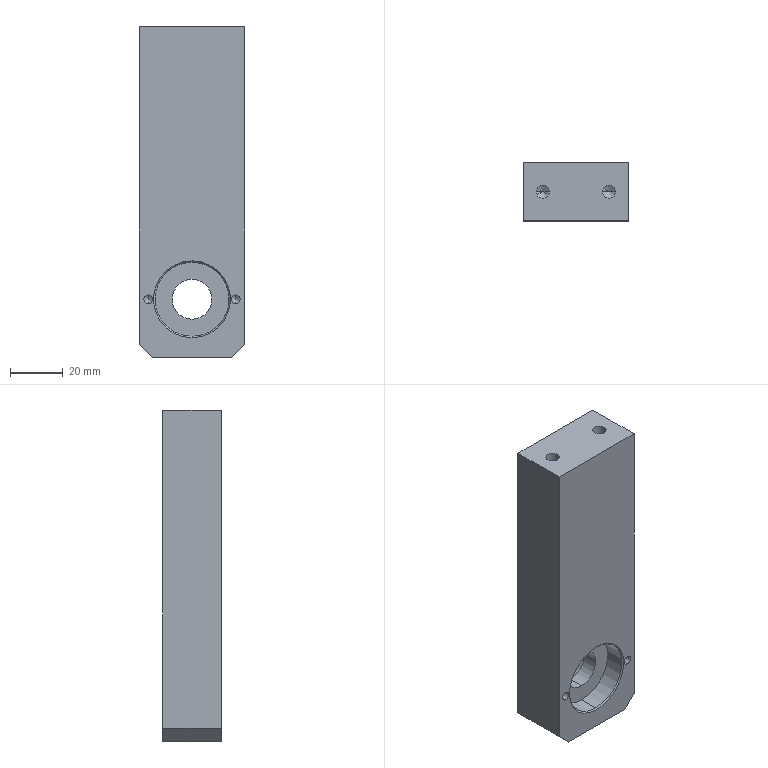Part | SolidWorks | features BaseBody 1 | 1 solid | 44 faces | box 40 x 22 x 125 mm | volume 97550 mm3 | cylinder 18 | cone 16 | plane 10 | commonest cylinder face diameters 3.3 x8 5 x4 28 x4 15 x2
STEP:
#1=CARTESIAN_POINT('',(13.755,11.9,-37.563));
#2=VERTEX_POINT('',#1);
#3=CARTESIAN_POINT('',(13.755,11.9,-34.263));
#4=VERTEX_POINT('',#3);
#5=CARTESIAN_POINT('',(13.755,11.9,-35.913));
#6=DIRECTION('',(0.,1.,0.));
#7=DIRECTION('',(0.,0.,1.));
#8=AXIS2_PLACEMENT_3D('',#5,#6,#7);
#9=CIRCLE('',#8,1.65);
#10=EDGE_CURVE('',#2,#4,#9,.T.);
#11=ORIENTED_EDGE('',*,*,#10,.F.);
#12=CARTESIAN_POINT('',(13.755,22.,-37.563));
#13=VERTEX_POINT('',#12);
#14=CARTESIAN_POINT('',(13.755,22.,-37.563));
#15=DIRECTION('',(0.,1.,0.));
#16=VECTOR('',#15,1000.);
#17=LINE('',#14,#16);
#18=EDGE_CURVE('',#2,#13,#17,.T.);
#19=ORIENTED_EDGE('',*,*,#18,.T.);
#20=CARTESIAN_POINT('',(13.755,22.,-34.263));
#21=VERTEX_POINT('',#20);
#22=CARTESIAN_POINT('',(13.755,22.,-35.913));
#23=DIRECTION('',(0.,1.,0.));
#24=DIRECTION('',(0.,0.,1.));
#25=AXIS2_PLACEMENT_3D('',#22,#23,#24);
#26=CIRCLE('',#25,1.65);
#27=EDGE_CURVE('',#13,#21,#26,.T.);
#28=ORIENTED_EDGE('',*,*,#27,.T.);
#29=CARTESIAN_POINT('',(13.755,22.,-34.263));
#30=DIRECTION('',(0.,1.,0.));
#31=VECTOR('',#30,1000.);
#32=LINE('',#29,#31);
#33=EDGE_CURVE('',#4,#21,#32,.T.);
#34=ORIENTED_EDGE('',*,*,#33,.F.);
#35=EDGE_LOOP('',(#11,#19,#28,#34));
#36=FACE_OUTER_BOUND('',#35,.T.);
#37=CARTESIAN_POINT('',(13.755,22.,-35.913));
#38=DIRECTION('',(0.,1.,0.));
#39=DIRECTION('',(0.,0.,1.));
#40=AXIS2_PLACEMENT_3D('',#37,#38,#39);
#41=CYLINDRICAL_SURFACE('',#40,1.65);
#42=ADVANCED_FACE('',(#36),#41,.F.);
#43=CARTESIAN_POINT('',(13.755,11.,-36.065));
#44=VERTEX_POINT('',#43);
#45=CARTESIAN_POINT('',(13.755,11.,-35.761));
#46=VERTEX_POINT('',#45);
#47=CARTESIAN_POINT('',(13.755,11.,-35.913));
#48=DIRECTION('',(0.,1.,0.));
#49=DIRECTION('',(0.,0.,1.));
#50=AXIS2_PLACEMENT_3D('',#47,#48,#49);
#51=CIRCLE('',#50,0.1521);
#52=EDGE_CURVE('',#44,#46,#51,.T.);
#53=ORIENTED_EDGE('',*,*,#52,.F.);
#54=CARTESIAN_POINT('',(13.755,11.9,-37.563));
#55=DIRECTION('',(0.,0.515,-0.8572));
#56=VECTOR('',#55,1000.);
#57=LINE('',#54,#56);
#58=EDGE_CURVE('',#44,#2,#57,.T.);
#59=ORIENTED_EDGE('',*,*,#58,.T.);
#60=ORIENTED_EDGE('',*,*,#10,.T.);
#61=CARTESIAN_POINT('',(13.755,11.9,-34.263));
#62=DIRECTION('',(0.,0.515,0.8572));
#63=VECTOR('',#62,1000.);
#64=LINE('',#61,#63);
#65=EDGE_CURVE('',#46,#4,#64,.T.);
#66=ORIENTED_EDGE('',*,*,#65,.F.);
#67=EDGE_LOOP('',(#53,#59,#60,#66));
#68=FACE_OUTER_BOUND('',#67,.T.);
#69=CARTESIAN_POINT('',(13.755,11.9,-35.913));
#70=DIRECTION('',(0.,1.,0.));
#71=DIRECTION('',(0.,0.,1.));
#72=AXIS2_PLACEMENT_3D('',#69,#70,#71);
#73=CONICAL_SURFACE('',#72,1.65,1.03);
#74=ADVANCED_FACE('',(#68),#73,.F.);
#75=CARTESIAN_POINT('',(-19.245,11.9,-37.563));
#76=VERTEX_POINT('',#75);
#77=CARTESIAN_POINT('',(-19.245,11.9,-34.263));
#78=VERTEX_POINT('',#77);
#79=CARTESIAN_POINT('',(-19.245,11.9,-35.913));
#80=DIRECTION('',(0.,1.,0.));
#81=DIRECTION('',(0.,0.,1.));
#82=AXIS2_PLACEMENT_3D('',#79,#80,#81);
#83=CIRCLE('',#82,1.65);
#84=EDGE_CURVE('',#76,#78,#83,.T.);
#85=ORIENTED_EDGE('',*,*,#84,.F.);
#86=CARTESIAN_POINT('',(-19.245,22.,-37.563));
#87=VERTEX_POINT('',#86);
#88=CARTESIAN_POINT('',(-19.245,22.,-37.563));
#89=DIRECTION('',(0.,1.,0.));
#90=VECTOR('',#89,1000.);
#91=LINE('',#88,#90);
#92=EDGE_CURVE('',#76,#87,#91,.T.);
#93=ORIENTED_EDGE('',*,*,#92,.T.);
#94=CARTESIAN_POINT('',(-19.245,22.,-34.263));
#95=VERTEX_POINT('',#94);
#96=CARTESIAN_POINT('',(-19.245,22.,-35.913));
#97=DIRECTION('',(0.,1.,0.));
#98=DIRECTION('',(0.,0.,1.));
#99=AXIS2_PLACEMENT_3D('',#96,#97,#98);
#100=CIRCLE('',#99,1.65);
#101=EDGE_CURVE('',#87,#95,#100,.T.);
#102=ORIENTED_EDGE('',*,*,#101,.T.);
#103=CARTESIAN_POINT('',(-19.245,22.,-34.263));
#104=DIRECTION('',(0.,1.,0.));
#105=VECTOR('',#104,1000.);
#106=LINE('',#103,#105);
#107=EDGE_CURVE('',#78,#95,#106,.T.);
#108=ORIENTED_EDGE('',*,*,#107,.F.);
#109=EDGE_LOOP('',(#85,#93,#102,#108));
#110=FACE_OUTER_BOUND('',#109,.T.);
#111=CARTESIAN_POINT('',(-19.245,22.,-35.913));
#112=DIRECTION('',(0.,1.,0.));
#113=DIRECTION('',(0.,0.,1.));
#114=AXIS2_PLACEMENT_3D('',#111,#112,#113);
#115=CYLINDRICAL_SURFACE('',#114,1.65);
#116=ADVANCED_FACE('',(#110),#115,.F.);
#117=CARTESIAN_POINT('',(-19.245,11.,-36.065));
#118=VERTEX_POINT('',#117);
#119=CARTESIAN_POINT('',(-19.245,11.,-35.761));
#120=VERTEX_POINT('',#119);
#121=CARTESIAN_POINT('',(-19.245,11.,-35.913));
#122=DIRECTION('',(0.,1.,0.));
#123=DIRECTION('',(0.,0.,1.));
#124=AXIS2_PLACEMENT_3D('',#121,#122,#123);
#125=CIRCLE('',#124,0.1521);
#126=EDGE_CURVE('',#118,#120,#125,.T.);
#127=ORIENTED_EDGE('',*,*,#126,.F.);
#128=CARTESIAN_POINT('',(-19.245,11.9,-37.563));
#129=DIRECTION('',(0.,0.515,-0.8572));
#130=VECTOR('',#129,1000.);
#131=LINE('',#128,#130);
#132=EDGE_CURVE('',#118,#76,#131,.T.);
#133=ORIENTED_EDGE('',*,*,#132,.T.);
#134=ORIENTED_EDGE('',*,*,#84,.T.);
#135=CARTESIAN_POINT('',(-19.245,11.9,-34.263));
#136=DIRECTION('',(0.,0.515,0.8572));
#137=VECTOR('',#136,1000.);
#138=LINE('',#135,#137);
#139=EDGE_CURVE('',#120,#78,#138,.T.);
#140=ORIENTED_EDGE('',*,*,#139,.F.);
#141=EDGE_LOOP('',(#127,#133,#134,#140));
#142=FACE_OUTER_BOUND('',#141,.T.);
#143=CARTESIAN_POINT('',(-19.245,11.9,-35.913));
#144=DIRECTION('',(0.,1.,0.));
#145=DIRECTION('',(0.,0.,1.));
#146=AXIS2_PLACEMENT_3D('',#143,#144,#145);
#147=CONICAL_SURFACE('',#146,1.65,1.03);
#148=ADVANCED_FACE('',(#142),#147,.F.);
#149=CARTESIAN_POINT('',(13.755,10.1,-34.263));
#150=VERTEX_POINT('',#149);
#151=CARTESIAN_POINT('',(13.755,10.1,-37.563));
#152=VERTEX_POINT('',#151);
#153=CARTESIAN_POINT('',(13.755,10.1,-35.913));
#154=DIRECTION('',(0.,-1.,0.));
#155=DIRECTION('',(0.,0.,-1.));
#156=AXIS2_PLACEMENT_3D('',#153,#154,#155);
#157=CIRCLE('',#156,1.65);
#158=EDGE_CURVE('',#150,#152,#157,.T.);
#159=ORIENTED_EDGE('',*,*,#158,.F.);
#160=CARTESIAN_POINT('',(13.755,0.,-34.263));
#161=VERTEX_POINT('',#160);
#162=CARTESIAN_POINT('',(13.755,0.,-34.263));
#163=DIRECTION('',(0.,-1.,0.));
#164=VECTOR('',#163,1000.);
#165=LINE('',#162,#164);
#166=EDGE_CURVE('',#150,#161,#165,.T.);
#167=ORIENTED_EDGE('',*,*,#166,.T.);
#168=CARTESIAN_POINT('',(13.755,0.,-37.563));
#169=VERTEX_POINT('',#168);
#170=CARTESIAN_POINT('',(13.755,0.,-35.913));
#171=DIRECTION('',(0.,-1.,0.));
#172=DIRECTION('',(0.,0.,-1.));
#173=AXIS2_PLACEMENT_3D('',#170,#171,#172);
#174=CIRCLE('',#173,1.65);
#175=EDGE_CURVE('',#161,#169,#174,.T.);
#176=ORIENTED_EDGE('',*,*,#175,.T.);
#177=CARTESIAN_POINT('',(13.755,0.,-37.563));
#178=DIRECTION('',(0.,-1.,0.));
#179=VECTOR('',#178,1000.);
#180=LINE('',#177,#179);
#181=EDGE_CURVE('',#152,#169,#180,.T.);
#182=ORIENTED_EDGE('',*,*,#181,.F.);
#183=EDGE_LOOP('',(#159,#167,#176,#182));
#184=FACE_OUTER_BOUND('',#183,.T.);
#185=CARTESIAN_POINT('',(13.755,0.,-35.913));
#186=DIRECTION('',(0.,-1.,0.));
#187=DIRECTION('',(0.,0.,-1.));
#188=AXIS2_PLACEMENT_3D('',#185,#186,#187);
#189=CYLINDRICAL_SURFACE('',#188,1.65);
#190=ADVANCED_FACE('',(#184),#189,.F.);
#191=ORIENTED_EDGE('',*,*,#52,.T.);
#192=CARTESIAN_POINT('',(13.755,10.1,-34.263));
#193=DIRECTION('',(0.,-0.515,0.8572));
#194=VECTOR('',#193,1000.);
#195=LINE('',#192,#194);
#196=EDGE_CURVE('',#46,#150,#195,.T.);
#197=ORIENTED_EDGE('',*,*,#196,.T.);
#198=ORIENTED_EDGE('',*,*,#158,.T.);
#199=CARTESIAN_POINT('',(13.755,10.1,-37.563));
#200=DIRECTION('',(0.,-0.515,-0.8572));
#201=VECTOR('',#200,1000.);
#202=LINE('',#199,#201);
#203=EDGE_CURVE('',#44,#152,#202,.T.);
#204=ORIENTED_EDGE('',*,*,#203,.F.);
#205=EDGE_LOOP('',(#191,#197,#198,#204));
#206=FACE_OUTER_BOUND('',#205,.T.);
#207=CARTESIAN_POINT('',(13.755,10.1,-35.913));
#208=DIRECTION('',(0.,-1.,0.));
#209=DIRECTION('',(0.,0.,-1.));
#210=AXIS2_PLACEMENT_3D('',#207,#208,#209);
#211=CONICAL_SURFACE('',#210,1.65,1.03);
#212=ADVANCED_FACE('',(#206),#211,.F.);
#213=CARTESIAN_POINT('',(-19.245,10.1,-34.263));
#214=VERTEX_POINT('',#213);
#215=CARTESIAN_POINT('',(-19.245,10.1,-37.563));
#216=VERTEX_POINT('',#215);
#217=CARTESIAN_POINT('',(-19.245,10.1,-35.913));
#218=DIRECTION('',(0.,-1.,0.));
#219=DIRECTION('',(0.,0.,-1.));
#220=AXIS2_PLACEMENT_3D('',#217,#218,#219);
#221=CIRCLE('',#220,1.65);
#222=EDGE_CURVE('',#214,#216,#221,.T.);
#223=ORIENTED_EDGE('',*,*,#222,.F.);
#224=CARTESIAN_POINT('',(-19.245,0.,-34.263));
#225=VERTEX_POINT('',#224);
#226=CARTESIAN_POINT('',(-19.245,0.,-34.263));
#227=DIRECTION('',(0.,-1.,0.));
#228=VECTOR('',#227,1000.);
#229=LINE('',#226,#228);
#230=EDGE_CURVE('',#214,#225,#229,.T.);
#231=ORIENTED_EDGE('',*,*,#230,.T.);
#232=CARTESIAN_POINT('',(-19.245,0.,-37.563));
#233=VERTEX_POINT('',#232);
#234=CARTESIAN_POINT('',(-19.245,0.,-35.913));
#235=DIRECTION('',(0.,-1.,0.));
#236=DIRECTION('',(0.,0.,-1.));
#237=AXIS2_PLACEMENT_3D('',#234,#235,#236);
#238=CIRCLE('',#237,1.65);
#239=EDGE_CURVE('',#225,#233,#238,.T.);
#240=ORIENTED_EDGE('',*,*,#239,.T.);
#241=CARTESIAN_POINT('',(-19.245,0.,-37.563));
#242=DIRECTION('',(0.,-1.,0.));
#243=VECTOR('',#242,1000.);
#244=LINE('',#241,#243);
#245=EDGE_CURVE('',#216,#233,#244,.T.);
#246=ORIENTED_EDGE('',*,*,#245,.F.);
#247=EDGE_LOOP('',(#223,#231,#240,#246));
#248=FACE_OUTER_BOUND('',#247,.T.);
#249=CARTESIAN_POINT('',(-19.245,0.,-35.913));
#250=DIRECTION('',(0.,-1.,0.));
#251=DIRECTION('',(0.,0.,-1.));
#252=AXIS2_PLACEMENT_3D('',#249,#250,#251);
#253=CYLINDRICAL_SURFACE('',#252,1.65);
#254=ADVANCED_FACE('',(#248),#253,.F.);
#255=ORIENTED_EDGE('',*,*,#126,.T.);
#256=CARTESIAN_POINT('',(-19.245,10.1,-34.263));
#257=DIRECTION('',(0.,-0.515,0.8572));
#258=VECTOR('',#257,1000.);
#259=LINE('',#256,#258);
#260=EDGE_CURVE('',#120,#214,#259,.T.);
#261=ORIENTED_EDGE('',*,*,#260,.T.);
#262=ORIENTED_EDGE('',*,*,#222,.T.);
#263=CARTESIAN_POINT('',(-19.245,10.1,-37.563));
#264=DIRECTION('',(0.,-0.515,-0.8572));
#265=VECTOR('',#264,1000.);
#266=LINE('',#263,#265);
#267=EDGE_CURVE('',#118,#216,#266,.T.);
#268=ORIENTED_EDGE('',*,*,#267,.F.);
#269=EDGE_LOOP('',(#255,#261,#262,#268));
#270=FACE_OUTER_BOUND('',#269,.T.);
#271=CARTESIAN_POINT('',(-19.245,10.1,-35.913));
#272=DIRECTION('',(0.,-1.,0.));
#273=DIRECTION('',(0.,0.,-1.));
#274=AXIS2_PLACEMENT_3D('',#271,#272,#273);
#275=CONICAL_SURFACE('',#274,1.65,1.03);
#276=ADVANCED_FACE('',(#270),#275,.F.);
#277=CARTESIAN_POINT('',(-2.745,0.5,-21.913));
#278=VERTEX_POINT('',#277);
#279=CARTESIAN_POINT('',(-2.745,0.5,-49.913));
#280=VERTEX_POINT('',#279);
#281=CARTESIAN_POINT('',(-2.745,0.5,-35.913));
#282=DIRECTION('',(0.,-1.,0.));
#283=DIRECTION('',(0.,0.,1.));
#284=AXIS2_PLACEMENT_3D('',#281,#282,#283);
#285=CIRCLE('',#284,14.);
#286=EDGE_CURVE('',#278,#280,#285,.T.);
#287=ORIENTED_EDGE('',*,*,#286,.F.);
#288=CARTESIAN_POINT('',(-2.745,0.,-21.413));
#289=VERTEX_POINT('',#288);
#290=CARTESIAN_POINT('',(-2.745,0.5,-21.913));
#291=DIRECTION('',(0.,-0.7071,0.7071));
#292=VECTOR('',#291,1000.);
#293=LINE('',#290,#292);
#294=EDGE_CURVE('',#278,#289,#293,.T.);
#295=ORIENTED_EDGE('',*,*,#294,.T.);
#296=CARTESIAN_POINT('',(-2.745,0.,-50.413));
#297=VERTEX_POINT('',#296);
#298=CARTESIAN_POINT('',(-2.745,0.,-35.913));
#299=DIRECTION('',(0.,1.,0.));
#300=DIRECTION('',(0.,0.,1.));
#301=AXIS2_PLACEMENT_3D('',#298,#299,#300);
#302=CIRCLE('',#301,14.5);
#303=EDGE_CURVE('',#297,#289,#302,.T.);
#304=ORIENTED_EDGE('',*,*,#303,.F.);
#305=CARTESIAN_POINT('',(-2.745,0.5,-49.913));
#306=DIRECTION('',(0.,-0.7071,-0.7071));
#307=VECTOR('',#306,1000.);
#308=LINE('',#305,#307);
#309=EDGE_CURVE('',#280,#297,#308,.T.);
#310=ORIENTED_EDGE('',*,*,#309,.F.);
#311=EDGE_LOOP('',(#287,#295,#304,#310));
#312=FACE_OUTER_BOUND('',#311,.T.);
#313=CARTESIAN_POINT('',(-2.745,0.5,-35.913));
#314=DIRECTION('',(0.,-1.,0.));
#315=DIRECTION('',(0.,0.,-1.));
#316=AXIS2_PLACEMENT_3D('',#313,#314,#315);
#317=CONICAL_SURFACE('',#316,14.,0.7854);
#318=ADVANCED_FACE('',(#312),#317,.F.);
#319=CARTESIAN_POINT('',(-2.745,21.5,-49.913));
#320=VERTEX_POINT('',#319);
#321=CARTESIAN_POINT('',(-2.745,21.5,-21.913));
#322=VERTEX_POINT('',#321);
#323=CARTESIAN_POINT('',(-2.745,21.5,-35.913));
#324=DIRECTION('',(0.,1.,0.));
#325=DIRECTION('',(0.,0.,1.));
#326=AXIS2_PLACEMENT_3D('',#323,#324,#325);
#327=CIRCLE('',#326,14.);
#328=EDGE_CURVE('',#320,#322,#327,.T.);
#329=ORIENTED_EDGE('',*,*,#328,.F.);
#330=CARTESIAN_POINT('',(-2.745,22.,-50.413));
#331=VERTEX_POINT('',#330);
#332=CARTESIAN_POINT('',(-2.745,21.5,-49.913));
#333=DIRECTION('',(0.,0.7071,-0.7071));
#334=VECTOR('',#333,1000.);
#335=LINE('',#332,#334);
#336=EDGE_CURVE('',#320,#331,#335,.T.);
#337=ORIENTED_EDGE('',*,*,#336,.T.);
#338=CARTESIAN_POINT('',(-2.745,22.,-21.413));
#339=VERTEX_POINT('',#338);
#340=CARTESIAN_POINT('',(-2.745,22.,-35.913));
#341=DIRECTION('',(0.,-1.,0.));
#342=DIRECTION('',(0.,0.,1.));
#343=AXIS2_PLACEMENT_3D('',#340,#341,#342);
#344=CIRCLE('',#343,14.5);
#345=EDGE_CURVE('',#339,#331,#344,.T.);
#346=ORIENTED_EDGE('',*,*,#345,.F.);
#347=CARTESIAN_POINT('',(-2.745,21.5,-21.913));
#348=DIRECTION('',(0.,0.7071,0.7071));
#349=VECTOR('',#348,1000.);
#350=LINE('',#347,#349);
#351=EDGE_CURVE('',#322,#339,#350,.T.);
#352=ORIENTED_EDGE('',*,*,#351,.F.);
#353=EDGE_LOOP('',(#329,#337,#346,#352));
#354=FACE_OUTER_BOUND('',#353,.T.);
#355=CARTESIAN_POINT('',(-2.745,21.5,-35.913));
#356=DIRECTION('',(0.,1.,0.));
#357=DIRECTION('',(0.,0.,1.));
#358=AXIS2_PLACEMENT_3D('',#355,#356,#357);
#359=CONICAL_SURFACE('',#358,14.,0.7854);
#360=ADVANCED_FACE('',(#354),#359,.F.);
#361=CARTESIAN_POINT('',(-2.745,8.,-21.913));
#362=VERTEX_POINT('',#361);
#363=CARTESIAN_POINT('',(-2.745,8.,-49.913));
#364=VERTEX_POINT('',#363);
#365=CARTESIAN_POINT('',(-2.745,8.,-35.913));
#366=DIRECTION('',(0.,-1.,0.));
#367=DIRECTION('',(0.,0.,-1.));
#368=AXIS2_PLACEMENT_3D('',#365,#366,#367);
#369=CIRCLE('',#368,14.);
#370=EDGE_CURVE('',#362,#364,#369,.T.);
#371=ORIENTED_EDGE('',*,*,#370,.F.);
#372=CARTESIAN_POINT('',(-2.745,8.,-21.913));
#373=DIRECTION('',(0.,-1.,0.));
#374=VECTOR('',#373,1000.);
#375=LINE('',#372,#374);
#376=EDGE_CURVE('',#362,#278,#375,.T.);
#377=ORIENTED_EDGE('',*,*,#376,.T.);
#378=ORIENTED_EDGE('',*,*,#286,.T.);
#379=CARTESIAN_POINT('',(-2.745,8.,-49.913));
#380=DIRECTION('',(0.,-1.,0.));
#381=VECTOR('',#380,1000.);
#382=LINE('',#379,#381);
#383=EDGE_CURVE('',#364,#280,#382,.T.);
#384=ORIENTED_EDGE('',*,*,#383,.F.);
#385=EDGE_LOOP('',(#371,#377,#378,#384));
#386=FACE_OUTER_BOUND('',#385,.T.);
#387=CARTESIAN_POINT('',(-2.745,8.,-35.913));
#388=DIRECTION('',(0.,-1.,0.));
#389=DIRECTION('',(0.,0.,-1.));
#390=AXIS2_PLACEMENT_3D('',#387,#388,#389);
#391=CYLINDRICAL_SURFACE('',#390,14.);
#392=ADVANCED_FACE('',(#386),#391,.F.);
#393=CARTESIAN_POINT('',(-17.745,11.,52.087));
#394=VERTEX_POINT('',#393);
#395=CARTESIAN_POINT('',(-12.745,11.,52.087));
#396=VERTEX_POINT('',#395);
#397=CARTESIAN_POINT('',(-15.245,11.,52.087));
#398=DIRECTION('',(0.,0.,1.));
#399=DIRECTION('',(1.,0.,0.));
#400=AXIS2_PLACEMENT_3D('',#397,#398,#399);
#401=CIRCLE('',#400,2.5);
#402=EDGE_CURVE('',#394,#396,#401,.T.);
#403=ORIENTED_EDGE('',*,*,#402,.F.);
#404=CARTESIAN_POINT('',(-17.745,11.,67.087));
#405=VERTEX_POINT('',#404);
#406=CARTESIAN_POINT('',(-17.745,11.,67.087));
#407=DIRECTION('',(0.,0.,1.));
#408=VECTOR('',#407,1000.);
#409=LINE('',#406,#408);
#410=EDGE_CURVE('',#394,#405,#409,.T.);
#411=ORIENTED_EDGE('',*,*,#410,.T.);
#412=CARTESIAN_POINT('',(-12.745,11.,67.087));
#413=VERTEX_POINT('',#412);
#414=CARTESIAN_POINT('',(-15.245,11.,67.087));
#415=DIRECTION('',(0.,0.,1.));
#416=DIRECTION('',(1.,0.,0.));
#417=AXIS2_PLACEMENT_3D('',#414,#415,#416);
#418=CIRCLE('',#417,2.5);
#419=EDGE_CURVE('',#405,#413,#418,.T.);
#420=ORIENTED_EDGE('',*,*,#419,.T.);
#421=CARTESIAN_POINT('',(-12.745,11.,67.087));
#422=DIRECTION('',(0.,0.,1.));
#423=VECTOR('',#422,1000.);
#424=LINE('',#421,#423);
#425=EDGE_CURVE('',#396,#413,#424,.T.);
#426=ORIENTED_EDGE('',*,*,#425,.F.);
#427=EDGE_LOOP('',(#403,#411,#420,#426));
#428=FACE_OUTER_BOUND('',#427,.T.);
#429=CARTESIAN_POINT('',(-15.245,11.,67.087));
#430=DIRECTION('',(0.,0.,1.));
#431=DIRECTION('',(1.,0.,0.));
#432=AXIS2_PLACEMENT_3D('',#429,#430,#431);
#433=CYLINDRICAL_SURFACE('',#432,2.5);
#434=ADVANCED_FACE('',(#428),#433,.F.);
#435=CARTESIAN_POINT('',(-15.245,11.,50.585));
#436=VERTEX_POINT('',#435);
#437=CARTESIAN_POINT('',(-12.745,11.,52.087));
#438=DIRECTION('',(0.8572,0.,0.515));
#439=VECTOR('',#438,1000.);
#440=LINE('',#437,#439);
#441=EDGE_CURVE('',#436,#396,#440,.T.);
#442=ORIENTED_EDGE('',*,*,#441,.F.);
#443=CARTESIAN_POINT('',(-17.745,11.,52.087));
#444=DIRECTION('',(-0.8572,0.,0.515));
#445=VECTOR('',#444,1000.);
#446=LINE('',#443,#445);
#447=EDGE_CURVE('',#436,#394,#446,.T.);
#448=ORIENTED_EDGE('',*,*,#447,.T.);
#449=ORIENTED_EDGE('',*,*,#402,.T.);
#450=EDGE_LOOP('',(#442,#448,#449));
#451=FACE_OUTER_BOUND('',#450,.T.);
#452=CARTESIAN_POINT('',(-15.245,11.,52.087));
#453=DIRECTION('',(0.,0.,1.));
#454=DIRECTION('',(1.,0.,0.));
#455=AXIS2_PLACEMENT_3D('',#452,#453,#454);
#456=CONICAL_SURFACE('',#455,2.5,1.03);
#457=ADVANCED_FACE('',(#451),#456,.F.);
#458=CARTESIAN_POINT('',(7.255,11.,52.087));
#459=VERTEX_POINT('',#458);
#460=CARTESIAN_POINT('',(12.255,11.,52.087));
#461=VERTEX_POINT('',#460);
#462=CARTESIAN_POINT('',(9.755,11.,52.087));
#463=DIRECTION('',(0.,0.,1.));
#464=DIRECTION('',(1.,0.,0.));
#465=AXIS2_PLACEMENT_3D('',#462,#463,#464);
#466=CIRCLE('',#465,2.5);
#467=EDGE_CURVE('',#459,#461,#466,.T.);
#468=ORIENTED_EDGE('',*,*,#467,.F.);
#469=CARTESIAN_POINT('',(7.255,11.,67.087));
#470=VERTEX_POINT('',#469);
#471=CARTESIAN_POINT('',(7.255,11.,67.087));
#472=DIRECTION('',(0.,0.,1.));
#473=VECTOR('',#472,1000.);
#474=LINE('',#471,#473);
#475=EDGE_CURVE('',#459,#470,#474,.T.);
#476=ORIENTED_EDGE('',*,*,#475,.T.);
#477=CARTESIAN_POINT('',(12.255,11.,67.087));
#478=VERTEX_POINT('',#477);
#479=CARTESIAN_POINT('',(9.755,11.,67.087));
#480=DIRECTION('',(0.,0.,1.));
#481=DIRECTION('',(1.,0.,0.));
#482=AXIS2_PLACEMENT_3D('',#479,#480,#481);
#483=CIRCLE('',#482,2.5);
#484=EDGE_CURVE('',#470,#478,#483,.T.);
#485=ORIENTED_EDGE('',*,*,#484,.T.);
#486=CARTESIAN_POINT('',(12.255,11.,67.087));
#487=DIRECTION('',(0.,0.,1.));
#488=VECTOR('',#487,1000.);
#489=LINE('',#486,#488);
#490=EDGE_CURVE('',#461,#478,#489,.T.);
#491=ORIENTED_EDGE('',*,*,#490,.F.);
#492=EDGE_LOOP('',(#468,#476,#485,#491));
#493=FACE_OUTER_BOUND('',#492,.T.);
#494=CARTESIAN_POINT('',(9.755,11.,67.087));
#495=DIRECTION('',(0.,0.,1.));
#496=DIRECTION('',(1.,0.,0.));
#497=AXIS2_PLACEMENT_3D('',#494,#495,#496);
#498=CYLINDRICAL_SURFACE('',#497,2.5);
#499=ADVANCED_FACE('',(#493),#498,.F.);
#500=CARTESIAN_POINT('',(9.755,11.,50.585));
#501=VERTEX_POINT('',#500);
#502=CARTESIAN_POINT('',(12.255,11.,52.087));
#503=DIRECTION('',(0.8572,0.,0.515));
#504=VECTOR('',#503,1000.);
#505=LINE('',#502,#504);
#506=EDGE_CURVE('',#501,#461,#505,.T.);
#507=ORIENTED_EDGE('',*,*,#506,.F.);
#508=CARTESIAN_POINT('',(7.255,11.,52.087));
#509=DIRECTION('',(-0.8572,0.,0.515));
#510=VECTOR('',#509,1000.);
#511=LINE('',#508,#510);
#512=EDGE_CURVE('',#501,#459,#511,.T.);
#513=ORIENTED_EDGE('',*,*,#512,.T.);
#514=ORIENTED_EDGE('',*,*,#467,.T.);
#515=EDGE_LOOP('',(#507,#513,#514));
#516=FACE_OUTER_BOUND('',#515,.T.);
#517=CARTESIAN_POINT('',(9.755,11.,52.087));
#518=DIRECTION('',(0.,0.,1.));
#519=DIRECTION('',(1.,0.,0.));
#520=AXIS2_PLACEMENT_3D('',#517,#518,#519);
#521=CONICAL_SURFACE('',#520,2.5,1.03);
#522=ADVANCED_FACE('',(#516),#521,.F.);
#523=CARTESIAN_POINT('',(-2.745,14.,-49.913));
#524=VERTEX_POINT('',#523);
#525=CARTESIAN_POINT('',(-2.745,14.,-21.913));
#526=VERTEX_POINT('',#525);
#527=CARTESIAN_POINT('',(-2.745,14.,-35.913));
#528=DIRECTION('',(0.,1.,0.));
#529=DIRECTION('',(0.,0.,1.));
#530=AXIS2_PLACEMENT_3D('',#527,#528,#529);
#531=CIRCLE('',#530,14.);
#532=EDGE_CURVE('',#524,#526,#531,.T.);
#533=ORIENTED_EDGE('',*,*,#532,.F.);
#534=CARTESIAN_POINT('',(-2.745,14.,-49.913));
#535=DIRECTION('',(0.,1.,0.));
#536=VECTOR('',#535,1000.);
#537=LINE('',#534,#536);
#538=EDGE_CURVE('',#524,#320,#537,.T.);
#539=ORIENTED_EDGE('',*,*,#538,.T.);
#540=ORIENTED_EDGE('',*,*,#328,.T.);
#541=CARTESIAN_POINT('',(-2.745,14.,-21.913));
#542=DIRECTION('',(0.,1.,0.));
#543=VECTOR('',#542,1000.);
#544=LINE('',#541,#543);
#545=EDGE_CURVE('',#526,#322,#544,.T.);
#546=ORIENTED_EDGE('',*,*,#545,.F.);
#547=EDGE_LOOP('',(#533,#539,#540,#546));
#548=FACE_OUTER_BOUND('',#547,.T.);
#549=CARTESIAN_POINT('',(-2.745,14.,-35.913));
#550=DIRECTION('',(0.,1.,0.));
#551=DIRECTION('',(0.,0.,1.));
#552=AXIS2_PLACEMENT_3D('',#549,#550,#551);
#553=CYLINDRICAL_SURFACE('',#552,14.);
#554=ADVANCED_FACE('',(#548),#553,.F.);
#555=CARTESIAN_POINT('',(-2.745,14.,-43.413));
#556=VERTEX_POINT('',#555);
#557=CARTESIAN_POINT('',(-2.745,14.,-28.413));
#558=VERTEX_POINT('',#557);
#559=CARTESIAN_POINT('',(-2.745,14.,-35.913));
#560=DIRECTION('',(0.,1.,0.));
#561=DIRECTION('',(0.,0.,1.));
#562=AXIS2_PLACEMENT_3D('',#559,#560,#561);
#563=CIRCLE('',#562,7.5);
#564=EDGE_CURVE('',#556,#558,#563,.T.);
#565=ORIENTED_EDGE('',*,*,#564,.T.);
#566=CARTESIAN_POINT('',(-2.745,8.,-28.413));
#567=VERTEX_POINT('',#566);
#568=CARTESIAN_POINT('',(-2.745,22.,-28.413));
#569=DIRECTION('',(0.,-1.,0.));
#570=VECTOR('',#569,1000.);
#571=LINE('',#568,#570);
#572=EDGE_CURVE('',#558,#567,#571,.T.);
#573=ORIENTED_EDGE('',*,*,#572,.T.);
#574=CARTESIAN_POINT('',(-2.745,8.,-43.413));
#575=VERTEX_POINT('',#574);
#576=CARTESIAN_POINT('',(-2.745,8.,-35.913));
#577=DIRECTION('',(0.,-1.,0.));
#578=DIRECTION('',(0.,0.,-1.));
#579=AXIS2_PLACEMENT_3D('',#576,#577,#578);
#580=CIRCLE('',#579,7.5);
#581=EDGE_CURVE('',#567,#575,#580,.T.);
#582=ORIENTED_EDGE('',*,*,#581,.T.);
#583=CARTESIAN_POINT('',(-2.745,22.,-43.413));
#584=DIRECTION('',(0.,-1.,0.));
#585=VECTOR('',#584,1000.);
#586=LINE('',#583,#585);
#587=EDGE_CURVE('',#556,#575,#586,.T.);
#588=ORIENTED_EDGE('',*,*,#587,.F.);
#589=EDGE_LOOP('',(#565,#573,#582,#588));
#590=FACE_OUTER_BOUND('',#589,.T.);
#591=CARTESIAN_POINT('',(-2.745,22.,-35.913));
#592=DIRECTION('',(0.,-1.,0.));
#593=DIRECTION('',(0.,0.,-1.));
#594=AXIS2_PLACEMENT_3D('',#591,#592,#593);
#595=CYLINDRICAL_SURFACE('',#594,7.5);
#596=ADVANCED_FACE('',(#590),#595,.F.);
#597=CARTESIAN_POINT('',(-2.745,8.,-35.913));
#598=DIRECTION('',(0.,-1.,0.));
#599=DIRECTION('',(0.,0.,-1.));
#600=AXIS2_PLACEMENT_3D('',#597,#598,#599);
#601=CIRCLE('',#600,7.5);
#602=EDGE_CURVE('',#575,#567,#601,.T.);
#603=ORIENTED_EDGE('',*,*,#602,.F.);
#604=ORIENTED_EDGE('',*,*,#581,.F.);
#605=EDGE_LOOP('',(#603,#604));
#606=FACE_BOUND('',#605,.T.);
#607=CARTESIAN_POINT('',(-2.745,8.,-35.913));
#608=DIRECTION('',(0.,-1.,0.));
#609=DIRECTION('',(0.,0.,-1.));
#610=AXIS2_PLACEMENT_3D('',#607,#608,#609);
#611=CIRCLE('',#610,14.);
#612=EDGE_CURVE('',#364,#362,#611,.T.);
#613=ORIENTED_EDGE('',*,*,#612,.T.);
#614=ORIENTED_EDGE('',*,*,#370,.T.);
#615=EDGE_LOOP('',(#613,#614));
#616=FACE_OUTER_BOUND('',#615,.T.);
#617=CARTESIAN_POINT('',(-2.745,8.,-35.913));
#618=DIRECTION('',(0.,-1.,0.));
#619=DIRECTION('',(0.,0.,-1.));
#620=AXIS2_PLACEMENT_3D('',#617,#618,#619);
#621=PLANE('',#620);
#622=ADVANCED_FACE('',(#606,#616),#621,.T.);
#623=CARTESIAN_POINT('',(-17.745,22.,-57.913));
#624=VERTEX_POINT('',#623);
#625=CARTESIAN_POINT('',(-22.745,22.,-52.913));
#626=VERTEX_POINT('',#625);
#627=CARTESIAN_POINT('',(-37.829,22.,-37.829));
#628=DIRECTION('',(-0.7071,0.,0.7071));
#629=VECTOR('',#628,1000.);
#630=LINE('',#627,#629);
#631=EDGE_CURVE('',#624,#626,#630,.T.);
#632=ORIENTED_EDGE('',*,*,#631,.F.);
#633=CARTESIAN_POINT('',(-17.745,0.,-57.913));
#634=VERTEX_POINT('',#633);
#635=CARTESIAN_POINT('',(-17.745,22.,-57.913));
#636=DIRECTION('',(0.,1.,0.));
#637=VECTOR('',#636,1000.);
#638=LINE('',#635,#637);
#639=EDGE_CURVE('',#634,#624,#638,.T.);
#640=ORIENTED_EDGE('',*,*,#639,.F.);
#641=CARTESIAN_POINT('',(-22.745,0.,-52.913));
#642=VERTEX_POINT('',#641);
#643=CARTESIAN_POINT('',(-22.745,0.,-52.913));
#644=DIRECTION('',(0.7071,0.,-0.7071));
#645=VECTOR('',#644,1000.);
#646=LINE('',#643,#645);
#647=EDGE_CURVE('',#642,#634,#646,.T.);
#648=ORIENTED_EDGE('',*,*,#647,.F.);
#649=CARTESIAN_POINT('',(-22.745,22.,-52.913));
#650=DIRECTION('',(0.,-1.,0.));
#651=VECTOR('',#650,1000.);
#652=LINE('',#649,#651);
#653=EDGE_CURVE('',#626,#642,#652,.T.);
#654=ORIENTED_EDGE('',*,*,#653,.F.);
#655=EDGE_LOOP('',(#632,#640,#648,#654));
#656=FACE_OUTER_BOUND('',#655,.T.);
#657=CARTESIAN_POINT('',(-22.745,22.,-52.913));
#658=DIRECTION('',(0.7071,0.,0.7071));
#659=DIRECTION('',(0.,-1.,0.));
#660=AXIS2_PLACEMENT_3D('',#657,#658,#659);
#661=PLANE('',#660);
#662=ADVANCED_FACE('',(#656),#661,.F.);
#663=CARTESIAN_POINT('',(17.255,22.,-52.913));
#664=VERTEX_POINT('',#663);
#665=CARTESIAN_POINT('',(12.255,22.,-57.913));
#666=VERTEX_POINT('',#665);
#667=CARTESIAN_POINT('',(35.084,22.,-35.084));
#668=DIRECTION('',(-0.7071,0.,-0.7071));
#669=VECTOR('',#668,1000.);
#670=LINE('',#667,#669);
#671=EDGE_CURVE('',#664,#666,#670,.T.);
#672=ORIENTED_EDGE('',*,*,#671,.F.);
#673=CARTESIAN_POINT('',(17.255,0.,-52.913));
#674=VERTEX_POINT('',#673);
#675=CARTESIAN_POINT('',(17.255,22.,-52.913));
#676=DIRECTION('',(0.,1.,0.));
#677=VECTOR('',#676,1000.);
#678=LINE('',#675,#677);
#679=EDGE_CURVE('',#674,#664,#678,.T.);
#680=ORIENTED_EDGE('',*,*,#679,.F.);
#681=CARTESIAN_POINT('',(12.255,0.,-57.913));
#682=VERTEX_POINT('',#681);
#683=CARTESIAN_POINT('',(12.255,0.,-57.913));
#684=DIRECTION('',(0.7071,0.,0.7071));
#685=VECTOR('',#684,1000.);
#686=LINE('',#683,#685);
#687=EDGE_CURVE('',#682,#674,#686,.T.);
#688=ORIENTED_EDGE('',*,*,#687,.F.);
#689=CARTESIAN_POINT('',(12.255,22.,-57.913));
#690=DIRECTION('',(0.,-1.,0.));
#691=VECTOR('',#690,1000.);
#692=LINE('',#689,#691);
#693=EDGE_CURVE('',#666,#682,#692,.T.);
#694=ORIENTED_EDGE('',*,*,#693,.F.);
#695=EDGE_LOOP('',(#672,#680,#688,#694));
#696=FACE_OUTER_BOUND('',#695,.T.);
#697=CARTESIAN_POINT('',(12.255,22.,-57.913));
#698=DIRECTION('',(-0.7071,0.,0.7071));
#699=DIRECTION('',(0.,1.,0.));
#700=AXIS2_PLACEMENT_3D('',#697,#698,#699);
#701=PLANE('',#700);
#702=ADVANCED_FACE('',(#696),#701,.F.);
#703=ORIENTED_EDGE('',*,*,#564,.F.);
#704=CARTESIAN_POINT('',(-2.745,14.,-35.913));
#705=DIRECTION('',(0.,1.,0.));
#706=DIRECTION('',(0.,0.,1.));
#707=AXIS2_PLACEMENT_3D('',#704,#705,#706);
#708=CIRCLE('',#707,7.5);
#709=EDGE_CURVE('',#558,#556,#708,.T.);
#710=ORIENTED_EDGE('',*,*,#709,.F.);
#711=EDGE_LOOP('',(#703,#710));
#712=FACE_BOUND('',#711,.T.);
#713=CARTESIAN_POINT('',(-2.745,14.,-35.913));
#714=DIRECTION('',(0.,1.,0.));
#715=DIRECTION('',(0.,0.,1.));
#716=AXIS2_PLACEMENT_3D('',#713,#714,#715);
#717=CIRCLE('',#716,14.);
#718=EDGE_CURVE('',#526,#524,#717,.T.);
#719=ORIENTED_EDGE('',*,*,#718,.T.);
#720=ORIENTED_EDGE('',*,*,#532,.T.);
#721=EDGE_LOOP('',(#719,#720));
#722=FACE_OUTER_BOUND('',#721,.T.);
#723=CARTESIAN_POINT('',(-2.745,14.,-35.913));
#724=DIRECTION('',(0.,1.,0.));
#725=DIRECTION('',(1.,0.,0.));
#726=AXIS2_PLACEMENT_3D('',#723,#724,#725);
#727=PLANE('',#726);
#728=ADVANCED_FACE('',(#712,#722),#727,.T.);
#729=CARTESIAN_POINT('',(-22.745,22.,-57.913));
#730=DIRECTION('',(-1.,0.,0.));
#731=VECTOR('',#730,1000.);
#732=LINE('',#729,#731);
#733=EDGE_CURVE('',#666,#624,#732,.T.);
#734=ORIENTED_EDGE('',*,*,#733,.F.);
#735=ORIENTED_EDGE('',*,*,#693,.T.);
#736=CARTESIAN_POINT('',(-22.745,0.,-57.913));
#737=DIRECTION('',(-1.,0.,0.));
#738=VECTOR('',#737,1000.);
#739=LINE('',#736,#738);
#740=EDGE_CURVE('',#682,#634,#739,.T.);
#741=ORIENTED_EDGE('',*,*,#740,.T.);
#742=ORIENTED_EDGE('',*,*,#639,.T.);
#743=EDGE_LOOP('',(#734,#735,#741,#742));
#744=FACE_OUTER_BOUND('',#743,.T.);
#745=CARTESIAN_POINT('',(-22.745,22.,-57.913));
#746=DIRECTION('',(0.,0.,1.));
#747=DIRECTION('',(1.,0.,0.));
#748=AXIS2_PLACEMENT_3D('',#745,#746,#747);
#749=PLANE('',#748);
#750=ADVANCED_FACE('',(#744),#749,.F.);
#751=CARTESIAN_POINT('',(17.255,0.,67.087));
#752=VERTEX_POINT('',#751);
#753=CARTESIAN_POINT('',(17.255,0.,-57.913));
#754=DIRECTION('',(0.,0.,-1.));
#755=VECTOR('',#754,1000.);
#756=LINE('',#753,#755);
#757=EDGE_CURVE('',#752,#674,#756,.T.);
#758=ORIENTED_EDGE('',*,*,#757,.T.);
#759=ORIENTED_EDGE('',*,*,#679,.T.);
#760=CARTESIAN_POINT('',(17.255,22.,67.087));
#761=VERTEX_POINT('',#760);
#762=CARTESIAN_POINT('',(17.255,22.,-57.913));
#763=DIRECTION('',(0.,0.,-1.));
#764=VECTOR('',#763,1000.);
#765=LINE('',#762,#764);
#766=EDGE_CURVE('',#761,#664,#765,.T.);
#767=ORIENTED_EDGE('',*,*,#766,.F.);
#768=CARTESIAN_POINT('',(17.255,22.,67.087));
#769=DIRECTION('',(0.,-1.,0.));
#770=VECTOR('',#769,1000.);
#771=LINE('',#768,#770);
#772=EDGE_CURVE('',#761,#752,#771,.T.);
#773=ORIENTED_EDGE('',*,*,#772,.T.);
#774=EDGE_LOOP('',(#758,#759,#767,#773));
#775=FACE_OUTER_BOUND('',#774,.T.);
#776=CARTESIAN_POINT('',(17.255,22.,-57.913));
#777=DIRECTION('',(-1.,0.,0.));
#778=DIRECTION('',(0.,1.,0.));
#779=AXIS2_PLACEMENT_3D('',#776,#777,#778);
#780=PLANE('',#779);
#781=ADVANCED_FACE('',(#775),#780,.F.);
#782=CARTESIAN_POINT('',(9.755,11.,67.087));
#783=DIRECTION('',(0.,0.,1.));
#784=DIRECTION('',(1.,0.,0.));
#785=AXIS2_PLACEMENT_3D('',#782,#783,#784);
#786=CIRCLE('',#785,2.5);
#787=EDGE_CURVE('',#478,#470,#786,.T.);
#788=ORIENTED_EDGE('',*,*,#787,.F.);
#789=ORIENTED_EDGE('',*,*,#484,.F.);
#790=EDGE_LOOP('',(#788,#789));
#791=FACE_BOUND('',#790,.T.);
#792=CARTESIAN_POINT('',(-15.245,11.,67.087));
#793=DIRECTION('',(0.,0.,1.));
#794=DIRECTION('',(1.,0.,0.));
#795=AXIS2_PLACEMENT_3D('',#792,#793,#794);
#796=CIRCLE('',#795,2.5);
#797=EDGE_CURVE('',#413,#405,#796,.T.);
#798=ORIENTED_EDGE('',*,*,#797,.F.);
#799=ORIENTED_EDGE('',*,*,#419,.F.);
#800=EDGE_LOOP('',(#798,#799));
#801=FACE_BOUND('',#800,.T.);
#802=CARTESIAN_POINT('',(-22.745,0.,67.087));
#803=VERTEX_POINT('',#802);
#804=CARTESIAN_POINT('',(-22.745,0.,67.087));
#805=DIRECTION('',(1.,0.,0.));
#806=VECTOR('',#805,1000.);
#807=LINE('',#804,#806);
#808=EDGE_CURVE('',#803,#752,#807,.T.);
#809=ORIENTED_EDGE('',*,*,#808,.T.);
#810=ORIENTED_EDGE('',*,*,#772,.F.);
#811=CARTESIAN_POINT('',(-22.745,22.,67.087));
#812=VERTEX_POINT('',#811);
#813=CARTESIAN_POINT('',(-22.745,22.,67.087));
#814=DIRECTION('',(1.,0.,0.));
#815=VECTOR('',#814,1000.);
#816=LINE('',#813,#815);
#817=EDGE_CURVE('',#812,#761,#816,.T.);
#818=ORIENTED_EDGE('',*,*,#817,.F.);
#819=CARTESIAN_POINT('',(-22.745,22.,67.087));
#820=DIRECTION('',(0.,-1.,0.));
#821=VECTOR('',#820,1000.);
#822=LINE('',#819,#821);
#823=EDGE_CURVE('',#812,#803,#822,.T.);
#824=ORIENTED_EDGE('',*,*,#823,.T.);
#825=EDGE_LOOP('',(#809,#810,#818,#824));
#826=FACE_OUTER_BOUND('',#825,.T.);
#827=CARTESIAN_POINT('',(-22.745,22.,67.087));
#828=DIRECTION('',(0.,0.,-1.));
#829=DIRECTION('',(0.,-1.,0.));
#830=AXIS2_PLACEMENT_3D('',#827,#828,#829);
#831=PLANE('',#830);
#832=ADVANCED_FACE('',(#791,#801,#826),#831,.F.);
#833=CARTESIAN_POINT('',(-22.745,22.,-57.913));
#834=DIRECTION('',(0.,0.,1.));
#835=VECTOR('',#834,1000.);
#836=LINE('',#833,#835);
#837=EDGE_CURVE('',#626,#812,#836,.T.);
#838=ORIENTED_EDGE('',*,*,#837,.F.);
#839=ORIENTED_EDGE('',*,*,#653,.T.);
#840=CARTESIAN_POINT('',(-22.745,0.,-57.913));
#841=DIRECTION('',(0.,0.,1.));
#842=VECTOR('',#841,1000.);
#843=LINE('',#840,#842);
#844=EDGE_CURVE('',#642,#803,#843,.T.);
#845=ORIENTED_EDGE('',*,*,#844,.T.);
#846=ORIENTED_EDGE('',*,*,#823,.F.);
#847=EDGE_LOOP('',(#838,#839,#845,#846));
#848=FACE_OUTER_BOUND('',#847,.T.);
#849=CARTESIAN_POINT('',(-22.745,22.,-57.913));
#850=DIRECTION('',(1.,0.,0.));
#851=DIRECTION('',(0.,0.,-1.));
#852=AXIS2_PLACEMENT_3D('',#849,#850,#851);
#853=PLANE('',#852);
#854=ADVANCED_FACE('',(#848),#853,.F.);
#855=ORIENTED_EDGE('',*,*,#303,.T.);
#856=CARTESIAN_POINT('',(-2.745,0.,-35.913));
#857=DIRECTION('',(0.,1.,0.));
#858=DIRECTION('',(0.,0.,1.));
#859=AXIS2_PLACEMENT_3D('',#856,#857,#858);
#860=CIRCLE('',#859,14.5);
#861=EDGE_CURVE('',#289,#297,#860,.T.);
#862=ORIENTED_EDGE('',*,*,#861,.T.);
#863=EDGE_LOOP('',(#855,#862));
#864=FACE_BOUND('',#863,.T.);
#865=CARTESIAN_POINT('',(-19.245,0.,-35.913));
#866=DIRECTION('',(0.,-1.,0.));
#867=DIRECTION('',(0.,0.,-1.));
#868=AXIS2_PLACEMENT_3D('',#865,#866,#867);
#869=CIRCLE('',#868,1.65);
#870=EDGE_CURVE('',#233,#225,#869,.T.);
#871=ORIENTED_EDGE('',*,*,#870,.F.);
#872=ORIENTED_EDGE('',*,*,#239,.F.);
#873=EDGE_LOOP('',(#871,#872));
#874=FACE_BOUND('',#873,.T.);
#875=CARTESIAN_POINT('',(13.755,0.,-35.913));
#876=DIRECTION('',(0.,-1.,0.));
#877=DIRECTION('',(0.,0.,-1.));
#878=AXIS2_PLACEMENT_3D('',#875,#876,#877);
#879=CIRCLE('',#878,1.65);
#880=EDGE_CURVE('',#169,#161,#879,.T.);
#881=ORIENTED_EDGE('',*,*,#880,.F.);
#882=ORIENTED_EDGE('',*,*,#175,.F.);
#883=EDGE_LOOP('',(#881,#882));
#884=FACE_BOUND('',#883,.T.);
#885=ORIENTED_EDGE('',*,*,#740,.F.);
#886=ORIENTED_EDGE('',*,*,#687,.T.);
#887=ORIENTED_EDGE('',*,*,#757,.F.);
#888=ORIENTED_EDGE('',*,*,#808,.F.);
#889=ORIENTED_EDGE('',*,*,#844,.F.);
#890=ORIENTED_EDGE('',*,*,#647,.T.);
#891=EDGE_LOOP('',(#885,#886,#887,#888,#889,#890));
#892=FACE_OUTER_BOUND('',#891,.T.);
#893=CARTESIAN_POINT('',(0.,0.,0.));
#894=DIRECTION('',(0.,1.,0.));
#895=DIRECTION('',(1.,0.,0.));
#896=AXIS2_PLACEMENT_3D('',#893,#894,#895);
#897=PLANE('',#896);
#898=ADVANCED_FACE('',(#864,#874,#884,#892),#897,.F.);
#899=ORIENTED_EDGE('',*,*,#345,.T.);
#900=CARTESIAN_POINT('',(-2.745,22.,-35.913));
#901=DIRECTION('',(0.,-1.,0.));
#902=DIRECTION('',(0.,0.,1.));
#903=AXIS2_PLACEMENT_3D('',#900,#901,#902);
#904=CIRCLE('',#903,14.5);
#905=EDGE_CURVE('',#331,#339,#904,.T.);
#906=ORIENTED_EDGE('',*,*,#905,.T.);
#907=EDGE_LOOP('',(#899,#906));
#908=FACE_BOUND('',#907,.T.);
#909=CARTESIAN_POINT('',(-19.245,22.,-35.913));
#910=DIRECTION('',(0.,1.,0.));
#911=DIRECTION('',(0.,0.,1.));
#912=AXIS2_PLACEMENT_3D('',#909,#910,#911);
#913=CIRCLE('',#912,1.65);
#914=EDGE_CURVE('',#95,#87,#913,.T.);
#915=ORIENTED_EDGE('',*,*,#914,.F.);
#916=ORIENTED_EDGE('',*,*,#101,.F.);
#917=EDGE_LOOP('',(#915,#916));
#918=FACE_BOUND('',#917,.T.);
#919=CARTESIAN_POINT('',(13.755,22.,-35.913));
#920=DIRECTION('',(0.,1.,0.));
#921=DIRECTION('',(0.,0.,1.));
#922=AXIS2_PLACEMENT_3D('',#919,#920,#921);
#923=CIRCLE('',#922,1.65);
#924=EDGE_CURVE('',#21,#13,#923,.T.);
#925=ORIENTED_EDGE('',*,*,#924,.F.);
#926=ORIENTED_EDGE('',*,*,#27,.F.);
#927=EDGE_LOOP('',(#925,#926));
#928=FACE_BOUND('',#927,.T.);
#929=ORIENTED_EDGE('',*,*,#766,.T.);
#930=ORIENTED_EDGE('',*,*,#671,.T.);
#931=ORIENTED_EDGE('',*,*,#733,.T.);
#932=ORIENTED_EDGE('',*,*,#631,.T.);
#933=ORIENTED_EDGE('',*,*,#837,.T.);
#934=ORIENTED_EDGE('',*,*,#817,.T.);
#935=EDGE_LOOP('',(#929,#930,#931,#932,#933,#934));
#936=FACE_OUTER_BOUND('',#935,.T.);
#937=CARTESIAN_POINT('',(0.,22.,0.));
#938=DIRECTION('',(0.,1.,0.));
#939=DIRECTION('',(1.,0.,0.));
#940=AXIS2_PLACEMENT_3D('',#937,#938,#939);
#941=PLANE('',#940);
#942=ADVANCED_FACE('',(#908,#918,#928,#936),#941,.T.);
#943=ORIENTED_EDGE('',*,*,#572,.F.);
#944=ORIENTED_EDGE('',*,*,#709,.T.);
#945=ORIENTED_EDGE('',*,*,#587,.T.);
#946=ORIENTED_EDGE('',*,*,#602,.T.);
#947=EDGE_LOOP('',(#943,#944,#945,#946));
#948=FACE_OUTER_BOUND('',#947,.T.);
#949=CARTESIAN_POINT('',(-2.745,22.,-35.913));
#950=DIRECTION('',(0.,-1.,0.));
#951=DIRECTION('',(0.,0.,-1.));
#952=AXIS2_PLACEMENT_3D('',#949,#950,#951);
#953=CYLINDRICAL_SURFACE('',#952,7.5);
#954=ADVANCED_FACE('',(#948),#953,.F.);
#955=ORIENTED_EDGE('',*,*,#538,.F.);
#956=ORIENTED_EDGE('',*,*,#718,.F.);
#957=ORIENTED_EDGE('',*,*,#545,.T.);
#958=CARTESIAN_POINT('',(-2.745,21.5,-35.913));
#959=DIRECTION('',(0.,1.,0.));
#960=DIRECTION('',(0.,0.,1.));
#961=AXIS2_PLACEMENT_3D('',#958,#959,#960);
#962=CIRCLE('',#961,14.);
#963=EDGE_CURVE('',#322,#320,#962,.T.);
#964=ORIENTED_EDGE('',*,*,#963,.T.);
#965=EDGE_LOOP('',(#955,#956,#957,#964));
#966=FACE_OUTER_BOUND('',#965,.T.);
#967=CARTESIAN_POINT('',(-2.745,14.,-35.913));
#968=DIRECTION('',(0.,1.,0.));
#969=DIRECTION('',(0.,0.,1.));
#970=AXIS2_PLACEMENT_3D('',#967,#968,#969);
#971=CYLINDRICAL_SURFACE('',#970,14.);
#972=ADVANCED_FACE('',(#966),#971,.F.);
#973=ORIENTED_EDGE('',*,*,#512,.F.);
#974=ORIENTED_EDGE('',*,*,#506,.T.);
#975=CARTESIAN_POINT('',(9.755,11.,52.087));
#976=DIRECTION('',(0.,0.,1.));
#977=DIRECTION('',(1.,0.,0.));
#978=AXIS2_PLACEMENT_3D('',#975,#976,#977);
#979=CIRCLE('',#978,2.5);
#980=EDGE_CURVE('',#461,#459,#979,.T.);
#981=ORIENTED_EDGE('',*,*,#980,.T.);
#982=EDGE_LOOP('',(#973,#974,#981));
#983=FACE_OUTER_BOUND('',#982,.T.);
#984=CARTESIAN_POINT('',(9.755,11.,52.087));
#985=DIRECTION('',(0.,0.,1.));
#986=DIRECTION('',(1.,0.,0.));
#987=AXIS2_PLACEMENT_3D('',#984,#985,#986);
#988=CONICAL_SURFACE('',#987,2.5,1.03);
#989=ADVANCED_FACE('',(#983),#988,.F.);
#990=ORIENTED_EDGE('',*,*,#475,.F.);
#991=ORIENTED_EDGE('',*,*,#980,.F.);
#992=ORIENTED_EDGE('',*,*,#490,.T.);
#993=ORIENTED_EDGE('',*,*,#787,.T.);
#994=EDGE_LOOP('',(#990,#991,#992,#993));
#995=FACE_OUTER_BOUND('',#994,.T.);
#996=CARTESIAN_POINT('',(9.755,11.,67.087));
#997=DIRECTION('',(0.,0.,1.));
#998=DIRECTION('',(1.,0.,0.));
#999=AXIS2_PLACEMENT_3D('',#996,#997,#998);
#1000=CYLINDRICAL_SURFACE('',#999,2.5);
#1001=ADVANCED_FACE('',(#995),#1000,.F.);
#1002=ORIENTED_EDGE('',*,*,#447,.F.);
#1003=ORIENTED_EDGE('',*,*,#441,.T.);
#1004=CARTESIAN_POINT('',(-15.245,11.,52.087));
#1005=DIRECTION('',(0.,0.,1.));
#1006=DIRECTION('',(1.,0.,0.));
#1007=AXIS2_PLACEMENT_3D('',#1004,#1005,#1006);
#1008=CIRCLE('',#1007,2.5);
#1009=EDGE_CURVE('',#396,#394,#1008,.T.);
#1010=ORIENTED_EDGE('',*,*,#1009,.T.);
#1011=EDGE_LOOP('',(#1002,#1003,#1010));
#1012=FACE_OUTER_BOUND('',#1011,.T.);
#1013=CARTESIAN_POINT('',(-15.245,11.,52.087));
#1014=DIRECTION('',(0.,0.,1.));
#1015=DIRECTION('',(1.,0.,0.));
#1016=AXIS2_PLACEMENT_3D('',#1013,#1014,#1015);
#1017=CONICAL_SURFACE('',#1016,2.5,1.03);
#1018=ADVANCED_FACE('',(#1012),#1017,.F.);
#1019=ORIENTED_EDGE('',*,*,#410,.F.);
#1020=ORIENTED_EDGE('',*,*,#1009,.F.);
#1021=ORIENTED_EDGE('',*,*,#425,.T.);
#1022=ORIENTED_EDGE('',*,*,#797,.T.);
#1023=EDGE_LOOP('',(#1019,#1020,#1021,#1022));
#1024=FACE_OUTER_BOUND('',#1023,.T.);
#1025=CARTESIAN_POINT('',(-15.245,11.,67.087));
#1026=DIRECTION('',(0.,0.,1.));
#1027=DIRECTION('',(1.,0.,0.));
#1028=AXIS2_PLACEMENT_3D('',#1025,#1026,#1027);
#1029=CYLINDRICAL_SURFACE('',#1028,2.5);
#1030=ADVANCED_FACE('',(#1024),#1029,.F.);
#1031=ORIENTED_EDGE('',*,*,#376,.F.);
#1032=ORIENTED_EDGE('',*,*,#612,.F.);
#1033=ORIENTED_EDGE('',*,*,#383,.T.);
#1034=CARTESIAN_POINT('',(-2.745,0.5,-35.913));
#1035=DIRECTION('',(0.,-1.,0.));
#1036=DIRECTION('',(0.,0.,1.));
#1037=AXIS2_PLACEMENT_3D('',#1034,#1035,#1036);
#1038=CIRCLE('',#1037,14.);
#1039=EDGE_CURVE('',#280,#278,#1038,.T.);
#1040=ORIENTED_EDGE('',*,*,#1039,.T.);
#1041=EDGE_LOOP('',(#1031,#1032,#1033,#1040));
#1042=FACE_OUTER_BOUND('',#1041,.T.);
#1043=CARTESIAN_POINT('',(-2.745,8.,-35.913));
#1044=DIRECTION('',(0.,-1.,0.));
#1045=DIRECTION('',(0.,0.,-1.));
#1046=AXIS2_PLACEMENT_3D('',#1043,#1044,#1045);
#1047=CYLINDRICAL_SURFACE('',#1046,14.);
#1048=ADVANCED_FACE('',(#1042),#1047,.F.);
#1049=ORIENTED_EDGE('',*,*,#336,.F.);
#1050=ORIENTED_EDGE('',*,*,#963,.F.);
#1051=ORIENTED_EDGE('',*,*,#351,.T.);
#1052=ORIENTED_EDGE('',*,*,#905,.F.);
#1053=EDGE_LOOP('',(#1049,#1050,#1051,#1052));
#1054=FACE_OUTER_BOUND('',#1053,.T.);
#1055=CARTESIAN_POINT('',(-2.745,21.5,-35.913));
#1056=DIRECTION('',(0.,1.,0.));
#1057=DIRECTION('',(0.,0.,1.));
#1058=AXIS2_PLACEMENT_3D('',#1055,#1056,#1057);
#1059=CONICAL_SURFACE('',#1058,14.,0.7854);
#1060=ADVANCED_FACE('',(#1054),#1059,.F.);
#1061=ORIENTED_EDGE('',*,*,#294,.F.);
#1062=ORIENTED_EDGE('',*,*,#1039,.F.);
#1063=ORIENTED_EDGE('',*,*,#309,.T.);
#1064=ORIENTED_EDGE('',*,*,#861,.F.);
#1065=EDGE_LOOP('',(#1061,#1062,#1063,#1064));
#1066=FACE_OUTER_BOUND('',#1065,.T.);
#1067=CARTESIAN_POINT('',(-2.745,0.5,-35.913));
#1068=DIRECTION('',(0.,-1.,0.));
#1069=DIRECTION('',(0.,0.,-1.));
#1070=AXIS2_PLACEMENT_3D('',#1067,#1068,#1069);
#1071=CONICAL_SURFACE('',#1070,14.,0.7854);
#1072=ADVANCED_FACE('',(#1066),#1071,.F.);
#1073=ORIENTED_EDGE('',*,*,#260,.F.);
#1074=CARTESIAN_POINT('',(-19.245,11.,-35.913));
#1075=DIRECTION('',(0.,1.,0.));
#1076=DIRECTION('',(0.,0.,1.));
#1077=AXIS2_PLACEMENT_3D('',#1074,#1075,#1076);
#1078=CIRCLE('',#1077,0.1521);
#1079=EDGE_CURVE('',#120,#118,#1078,.T.);
#1080=ORIENTED_EDGE('',*,*,#1079,.T.);
#1081=ORIENTED_EDGE('',*,*,#267,.T.);
#1082=CARTESIAN_POINT('',(-19.245,10.1,-35.913));
#1083=DIRECTION('',(0.,-1.,0.));
#1084=DIRECTION('',(0.,0.,-1.));
#1085=AXIS2_PLACEMENT_3D('',#1082,#1083,#1084);
#1086=CIRCLE('',#1085,1.65);
#1087=EDGE_CURVE('',#216,#214,#1086,.T.);
#1088=ORIENTED_EDGE('',*,*,#1087,.T.);
#1089=EDGE_LOOP('',(#1073,#1080,#1081,#1088));
#1090=FACE_OUTER_BOUND('',#1089,.T.);
#1091=CARTESIAN_POINT('',(-19.245,10.1,-35.913));
#1092=DIRECTION('',(0.,-1.,0.));
#1093=DIRECTION('',(0.,0.,-1.));
#1094=AXIS2_PLACEMENT_3D('',#1091,#1092,#1093);
#1095=CONICAL_SURFACE('',#1094,1.65,1.03);
#1096=ADVANCED_FACE('',(#1090),#1095,.F.);
#1097=ORIENTED_EDGE('',*,*,#230,.F.);
#1098=ORIENTED_EDGE('',*,*,#1087,.F.);
#1099=ORIENTED_EDGE('',*,*,#245,.T.);
#1100=ORIENTED_EDGE('',*,*,#870,.T.);
#1101=EDGE_LOOP('',(#1097,#1098,#1099,#1100));
#1102=FACE_OUTER_BOUND('',#1101,.T.);
#1103=CARTESIAN_POINT('',(-19.245,0.,-35.913));
#1104=DIRECTION('',(0.,-1.,0.));
#1105=DIRECTION('',(0.,0.,-1.));
#1106=AXIS2_PLACEMENT_3D('',#1103,#1104,#1105);
#1107=CYLINDRICAL_SURFACE('',#1106,1.65);
#1108=ADVANCED_FACE('',(#1102),#1107,.F.);
#1109=ORIENTED_EDGE('',*,*,#196,.F.);
#1110=CARTESIAN_POINT('',(13.755,11.,-35.913));
#1111=DIRECTION('',(0.,1.,0.));
#1112=DIRECTION('',(0.,0.,1.));
#1113=AXIS2_PLACEMENT_3D('',#1110,#1111,#1112);
#1114=CIRCLE('',#1113,0.1521);
#1115=EDGE_CURVE('',#46,#44,#1114,.T.);
#1116=ORIENTED_EDGE('',*,*,#1115,.T.);
#1117=ORIENTED_EDGE('',*,*,#203,.T.);
#1118=CARTESIAN_POINT('',(13.755,10.1,-35.913));
#1119=DIRECTION('',(0.,-1.,0.));
#1120=DIRECTION('',(0.,0.,-1.));
#1121=AXIS2_PLACEMENT_3D('',#1118,#1119,#1120);
#1122=CIRCLE('',#1121,1.65);
#1123=EDGE_CURVE('',#152,#150,#1122,.T.);
#1124=ORIENTED_EDGE('',*,*,#1123,.T.);
#1125=EDGE_LOOP('',(#1109,#1116,#1117,#1124));
#1126=FACE_OUTER_BOUND('',#1125,.T.);
#1127=CARTESIAN_POINT('',(13.755,10.1,-35.913));
#1128=DIRECTION('',(0.,-1.,0.));
#1129=DIRECTION('',(0.,0.,-1.));
#1130=AXIS2_PLACEMENT_3D('',#1127,#1128,#1129);
#1131=CONICAL_SURFACE('',#1130,1.65,1.03);
#1132=ADVANCED_FACE('',(#1126),#1131,.F.);
#1133=ORIENTED_EDGE('',*,*,#166,.F.);
#1134=ORIENTED_EDGE('',*,*,#1123,.F.);
#1135=ORIENTED_EDGE('',*,*,#181,.T.);
#1136=ORIENTED_EDGE('',*,*,#880,.T.);
#1137=EDGE_LOOP('',(#1133,#1134,#1135,#1136));
#1138=FACE_OUTER_BOUND('',#1137,.T.);
#1139=CARTESIAN_POINT('',(13.755,0.,-35.913));
#1140=DIRECTION('',(0.,-1.,0.));
#1141=DIRECTION('',(0.,0.,-1.));
#1142=AXIS2_PLACEMENT_3D('',#1139,#1140,#1141);
#1143=CYLINDRICAL_SURFACE('',#1142,1.65);
#1144=ADVANCED_FACE('',(#1138),#1143,.F.);
#1145=ORIENTED_EDGE('',*,*,#132,.F.);
#1146=ORIENTED_EDGE('',*,*,#1079,.F.);
#1147=ORIENTED_EDGE('',*,*,#139,.T.);
#1148=CARTESIAN_POINT('',(-19.245,11.9,-35.913));
#1149=DIRECTION('',(0.,1.,0.));
#1150=DIRECTION('',(0.,0.,1.));
#1151=AXIS2_PLACEMENT_3D('',#1148,#1149,#1150);
#1152=CIRCLE('',#1151,1.65);
#1153=EDGE_CURVE('',#78,#76,#1152,.T.);
#1154=ORIENTED_EDGE('',*,*,#1153,.T.);
#1155=EDGE_LOOP('',(#1145,#1146,#1147,#1154));
#1156=FACE_OUTER_BOUND('',#1155,.T.);
#1157=CARTESIAN_POINT('',(-19.245,11.9,-35.913));
#1158=DIRECTION('',(0.,1.,0.));
#1159=DIRECTION('',(0.,0.,1.));
#1160=AXIS2_PLACEMENT_3D('',#1157,#1158,#1159);
#1161=CONICAL_SURFACE('',#1160,1.65,1.03);
#1162=ADVANCED_FACE('',(#1156),#1161,.F.);
#1163=ORIENTED_EDGE('',*,*,#92,.F.);
#1164=ORIENTED_EDGE('',*,*,#1153,.F.);
#1165=ORIENTED_EDGE('',*,*,#107,.T.);
#1166=ORIENTED_EDGE('',*,*,#914,.T.);
#1167=EDGE_LOOP('',(#1163,#1164,#1165,#1166));
#1168=FACE_OUTER_BOUND('',#1167,.T.);
#1169=CARTESIAN_POINT('',(-19.245,22.,-35.913));
#1170=DIRECTION('',(0.,1.,0.));
#1171=DIRECTION('',(0.,0.,1.));
#1172=AXIS2_PLACEMENT_3D('',#1169,#1170,#1171);
#1173=CYLINDRICAL_SURFACE('',#1172,1.65);
#1174=ADVANCED_FACE('',(#1168),#1173,.F.);
#1175=ORIENTED_EDGE('',*,*,#58,.F.);
#1176=ORIENTED_EDGE('',*,*,#1115,.F.);
#1177=ORIENTED_EDGE('',*,*,#65,.T.);
#1178=CARTESIAN_POINT('',(13.755,11.9,-35.913));
#1179=DIRECTION('',(0.,1.,0.));
#1180=DIRECTION('',(0.,0.,1.));
#1181=AXIS2_PLACEMENT_3D('',#1178,#1179,#1180);
#1182=CIRCLE('',#1181,1.65);
#1183=EDGE_CURVE('',#4,#2,#1182,.T.);
#1184=ORIENTED_EDGE('',*,*,#1183,.T.);
#1185=EDGE_LOOP('',(#1175,#1176,#1177,#1184));
#1186=FACE_OUTER_BOUND('',#1185,.T.);
#1187=CARTESIAN_POINT('',(13.755,11.9,-35.913));
#1188=DIRECTION('',(0.,1.,0.));
#1189=DIRECTION('',(0.,0.,1.));
#1190=AXIS2_PLACEMENT_3D('',#1187,#1188,#1189);
#1191=CONICAL_SURFACE('',#1190,1.65,1.03);
#1192=ADVANCED_FACE('',(#1186),#1191,.F.);
#1193=ORIENTED_EDGE('',*,*,#18,.F.);
#1194=ORIENTED_EDGE('',*,*,#1183,.F.);
#1195=ORIENTED_EDGE('',*,*,#33,.T.);
#1196=ORIENTED_EDGE('',*,*,#924,.T.);
#1197=EDGE_LOOP('',(#1193,#1194,#1195,#1196));
#1198=FACE_OUTER_BOUND('',#1197,.T.);
#1199=CARTESIAN_POINT('',(13.755,22.,-35.913));
#1200=DIRECTION('',(0.,1.,0.));
#1201=DIRECTION('',(0.,0.,1.));
#1202=AXIS2_PLACEMENT_3D('',#1199,#1200,#1201);
#1203=CYLINDRICAL_SURFACE('',#1202,1.65);
#1204=ADVANCED_FACE('',(#1198),#1203,.F.);
#1205=CLOSED_SHELL('',(#42,#74,#116,#148,#190,#212,#254,#276,#318,#360,#392,#434,#457,#499,#522,#554,#596,#622,#662,#702,#728,#750,#781,#832,#854,#898,#942,#954,#972,#989,#1001,#1018,#1030,#1048,#1060,#1072,#1096,#1108,#1132,#1144,#1162,#1174,#1192,#1204));
#1206=MANIFOLD_SOLID_BREP('',#1205);
#1207=CARTESIAN_POINT('',(0.,0.,0.));
#1208=DIRECTION('',(0.,0.,1.));
#1209=DIRECTION('',(1.,0.,0.));
#1210=AXIS2_PLACEMENT_3D('',#1207,#1208,#1209);
#1211=(LENGTH_UNIT()NAMED_UNIT(*)SI_UNIT(.MILLI.,.METRE.));
#1212=UNCERTAINTY_MEASURE_WITH_UNIT(LENGTH_MEASURE(0.00001),#1211,'','');
#1213=(NAMED_UNIT(*)PLANE_ANGLE_UNIT()SI_UNIT($,.RADIAN.));
#1214=(NAMED_UNIT(*)SI_UNIT($,.STERADIAN.)SOLID_ANGLE_UNIT());
#1215=(GEOMETRIC_REPRESENTATION_CONTEXT(3)GLOBAL_UNCERTAINTY_ASSIGNED_CONTEXT((#1212))GLOBAL_UNIT_ASSIGNED_CONTEXT((#1211,#1213,#1214))REPRESENTATION_CONTEXT('',''));
#1216=ADVANCED_BREP_SHAPE_REPRESENTATION('',(#1206,#1210),#1215);